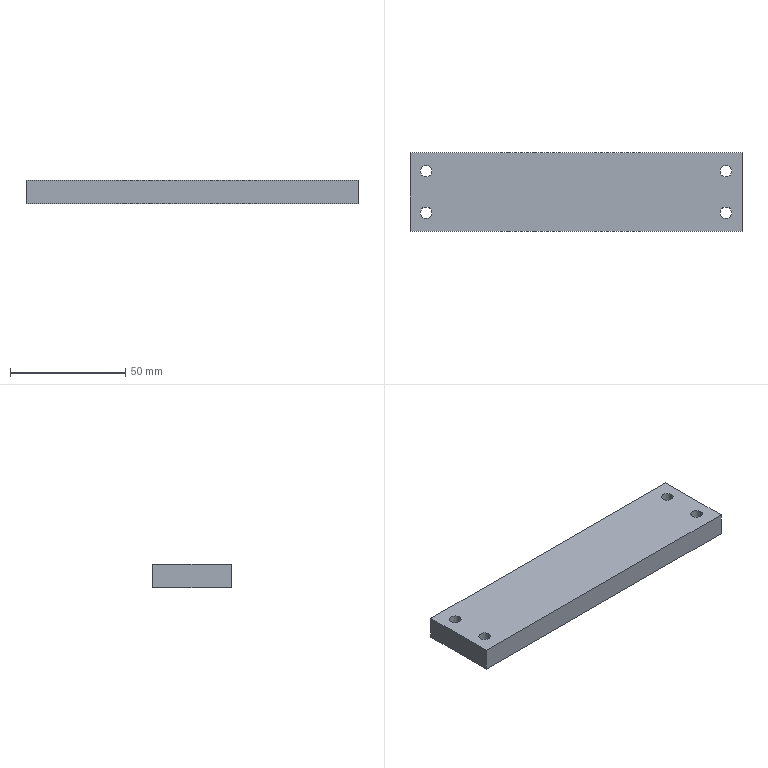Part | STEP file | Light curtain | 1 solid | 14 faces | box 144 x 34 x 10 mm | volume 48175 mm3 | cylinder 8 | plane 6 | commonest cylinder face diameters 5 x8
STEP:
#1=CARTESIAN_POINT('',(0.,0.,0.));
#2=DIRECTION('',(0.,0.,1.));
#3=DIRECTION('',(1.,0.,0.));
#4=AXIS2_PLACEMENT_3D('',#1,#2,#3);
#5=CARTESIAN_POINT('',(62.5,-9.,10.));
#6=VERTEX_POINT('',#5);
#7=CARTESIAN_POINT('',(62.5,-9.,0.));
#8=VERTEX_POINT('',#7);
#9=CARTESIAN_POINT('',(62.5,-9.,10.));
#10=DIRECTION('',(0.,0.,-1.));
#11=VECTOR('',#10,1.);
#12=LINE('',#9,#11);
#13=CARTESIAN_POINT('',(65.,-9.,10.));
#14=DIRECTION('',(0.,0.,-1.));
#15=DIRECTION('',(-1.,0.,0.));
#16=AXIS2_PLACEMENT_3D('',#13,#14,#15);
#17=CYLINDRICAL_SURFACE('',#16,2.5);
#18=CARTESIAN_POINT('',(6.283,0.));
#19=DIRECTION('',(0.,1.));
#20=VECTOR('',#19,1.);
#21=LINE('',#18,#20);
#22=(GEOMETRIC_REPRESENTATION_CONTEXT(2)PARAMETRIC_REPRESENTATION_CONTEXT()REPRESENTATION_CONTEXT('',''));
#23=DEFINITIONAL_REPRESENTATION('',(#21),#22);
#24=PCURVE('',#17,#23);
#25=CARTESIAN_POINT('',(65.,-9.,10.));
#26=DIRECTION('',(0.,0.,-1.));
#27=DIRECTION('',(-1.,0.,0.));
#28=AXIS2_PLACEMENT_3D('',#25,#26,#27);
#29=CYLINDRICAL_SURFACE('',#28,2.5);
#30=CARTESIAN_POINT('',(0.,0.));
#31=DIRECTION('',(0.,1.));
#32=VECTOR('',#31,1.);
#33=LINE('',#30,#32);
#34=(GEOMETRIC_REPRESENTATION_CONTEXT(2)PARAMETRIC_REPRESENTATION_CONTEXT()REPRESENTATION_CONTEXT('',''));
#35=DEFINITIONAL_REPRESENTATION('',(#33),#34);
#36=PCURVE('',#29,#35);
#37=SURFACE_CURVE('',#12,(#24,#36),.PCURVE_S1.);
#38=EDGE_CURVE('',#6,#8,#37,.T.);
#39=ORIENTED_EDGE('',*,*,#38,.T.);
#40=CARTESIAN_POINT('',(67.5,-9.,0.));
#41=VERTEX_POINT('',#40);
#42=CARTESIAN_POINT('',(65.,-9.,0.));
#43=DIRECTION('',(0.,0.,1.));
#44=DIRECTION('',(-1.,0.,0.));
#45=AXIS2_PLACEMENT_3D('',#42,#43,#44);
#46=CIRCLE('',#45,2.5);
#47=CARTESIAN_POINT('',(6.283,10.));
#48=DIRECTION('',(-1.,0.));
#49=VECTOR('',#48,1.);
#50=LINE('',#47,#49);
#51=(GEOMETRIC_REPRESENTATION_CONTEXT(2)PARAMETRIC_REPRESENTATION_CONTEXT()REPRESENTATION_CONTEXT('',''));
#52=DEFINITIONAL_REPRESENTATION('',(#50),#51);
#53=PCURVE('',#17,#52);
#54=CARTESIAN_POINT('',(72.,-17.,0.));
#55=DIRECTION('',(0.,0.,1.));
#56=DIRECTION('',(1.,0.,0.));
#57=AXIS2_PLACEMENT_3D('',#54,#55,#56);
#58=PLANE('',#57);
#59=CARTESIAN_POINT('',(-7.,8.));
#60=DIRECTION('',(-1.,0.));
#61=AXIS2_PLACEMENT_2D('',#59,#60);
#62=CIRCLE('',#61,2.5);
#63=(GEOMETRIC_REPRESENTATION_CONTEXT(2)PARAMETRIC_REPRESENTATION_CONTEXT()REPRESENTATION_CONTEXT('',''));
#64=DEFINITIONAL_REPRESENTATION('',(#62),#63);
#65=PCURVE('',#58,#64);
#66=SURFACE_CURVE('',#46,(#53,#65),.PCURVE_S1.);
#67=EDGE_CURVE('',#8,#41,#66,.T.);
#68=ORIENTED_EDGE('',*,*,#67,.T.);
#69=CARTESIAN_POINT('',(67.5,-9.,10.));
#70=VERTEX_POINT('',#69);
#71=CARTESIAN_POINT('',(67.5,-9.,10.));
#72=DIRECTION('',(0.,0.,-1.));
#73=VECTOR('',#72,1.);
#74=LINE('',#71,#73);
#75=CARTESIAN_POINT('',(3.142,0.));
#76=DIRECTION('',(0.,1.));
#77=VECTOR('',#76,1.);
#78=LINE('',#75,#77);
#79=(GEOMETRIC_REPRESENTATION_CONTEXT(2)PARAMETRIC_REPRESENTATION_CONTEXT()REPRESENTATION_CONTEXT('',''));
#80=DEFINITIONAL_REPRESENTATION('',(#78),#79);
#81=PCURVE('',#17,#80);
#82=CARTESIAN_POINT('',(3.142,0.));
#83=DIRECTION('',(0.,1.));
#84=VECTOR('',#83,1.);
#85=LINE('',#82,#84);
#86=(GEOMETRIC_REPRESENTATION_CONTEXT(2)PARAMETRIC_REPRESENTATION_CONTEXT()REPRESENTATION_CONTEXT('',''));
#87=DEFINITIONAL_REPRESENTATION('',(#85),#86);
#88=PCURVE('',#29,#87);
#89=SURFACE_CURVE('',#74,(#81,#88),.PCURVE_S1.);
#90=EDGE_CURVE('',#70,#41,#89,.T.);
#91=ORIENTED_EDGE('',*,*,#90,.F.);
#92=CARTESIAN_POINT('',(65.,-9.,10.));
#93=DIRECTION('',(0.,0.,-1.));
#94=DIRECTION('',(-1.,0.,0.));
#95=AXIS2_PLACEMENT_3D('',#92,#93,#94);
#96=CIRCLE('',#95,2.5);
#97=CARTESIAN_POINT('',(0.,0.));
#98=DIRECTION('',(1.,0.));
#99=VECTOR('',#98,1.);
#100=LINE('',#97,#99);
#101=(GEOMETRIC_REPRESENTATION_CONTEXT(2)PARAMETRIC_REPRESENTATION_CONTEXT()REPRESENTATION_CONTEXT('',''));
#102=DEFINITIONAL_REPRESENTATION('',(#100),#101);
#103=PCURVE('',#17,#102);
#104=CARTESIAN_POINT('',(72.,-17.,10.));
#105=DIRECTION('',(0.,0.,1.));
#106=DIRECTION('',(1.,0.,0.));
#107=AXIS2_PLACEMENT_3D('',#104,#105,#106);
#108=PLANE('',#107);
#109=CARTESIAN_POINT('',(-9.5,8.));
#110=CARTESIAN_POINT('',(-9.5,12.33));
#111=CARTESIAN_POINT('',(-5.75,10.165));
#112=CARTESIAN_POINT('',(-2.,8.));
#113=CARTESIAN_POINT('',(-5.75,5.835));
#114=CARTESIAN_POINT('',(-9.5,3.67));
#115=CARTESIAN_POINT('',(-9.5,8.));
#116=(BOUNDED_CURVE()B_SPLINE_CURVE(2,(#109,#110,#111,#112,#113,#114,#115),.UNSPECIFIED.,.T.,.F.)B_SPLINE_CURVE_WITH_KNOTS((1,2,2,2,2,1),(-2.094,0.,2.094,4.189,6.283,8.378),.UNSPECIFIED.)CURVE()GEOMETRIC_REPRESENTATION_ITEM()RATIONAL_B_SPLINE_CURVE((1.,0.5,1.,0.5,1.,0.5,1.))REPRESENTATION_ITEM(''));
#117=(GEOMETRIC_REPRESENTATION_CONTEXT(2)PARAMETRIC_REPRESENTATION_CONTEXT()REPRESENTATION_CONTEXT('',''));
#118=DEFINITIONAL_REPRESENTATION('',(#116),#117);
#119=PCURVE('',#108,#118);
#120=SURFACE_CURVE('',#96,(#103,#119),.PCURVE_S1.);
#121=EDGE_CURVE('',#70,#6,#120,.T.);
#122=ORIENTED_EDGE('',*,*,#121,.T.);
#123=EDGE_LOOP('',(#39,#68,#91,#122));
#124=FACE_BOUND('',#123,.F.);
#125=ADVANCED_FACE('',(#124),#17,.F.);
#126=CARTESIAN_POINT('',(62.5,9.,10.));
#127=VERTEX_POINT('',#126);
#128=CARTESIAN_POINT('',(62.5,9.,0.));
#129=VERTEX_POINT('',#128);
#130=CARTESIAN_POINT('',(62.5,9.,10.));
#131=DIRECTION('',(0.,0.,-1.));
#132=VECTOR('',#131,1.);
#133=LINE('',#130,#132);
#134=CARTESIAN_POINT('',(65.,9.,10.));
#135=DIRECTION('',(0.,0.,-1.));
#136=DIRECTION('',(-1.,0.,0.));
#137=AXIS2_PLACEMENT_3D('',#134,#135,#136);
#138=CYLINDRICAL_SURFACE('',#137,2.5);
#139=CARTESIAN_POINT('',(6.283,0.));
#140=DIRECTION('',(0.,1.));
#141=VECTOR('',#140,1.);
#142=LINE('',#139,#141);
#143=(GEOMETRIC_REPRESENTATION_CONTEXT(2)PARAMETRIC_REPRESENTATION_CONTEXT()REPRESENTATION_CONTEXT('',''));
#144=DEFINITIONAL_REPRESENTATION('',(#142),#143);
#145=PCURVE('',#138,#144);
#146=CARTESIAN_POINT('',(65.,9.,10.));
#147=DIRECTION('',(0.,0.,-1.));
#148=DIRECTION('',(-1.,0.,0.));
#149=AXIS2_PLACEMENT_3D('',#146,#147,#148);
#150=CYLINDRICAL_SURFACE('',#149,2.5);
#151=CARTESIAN_POINT('',(0.,0.));
#152=DIRECTION('',(0.,1.));
#153=VECTOR('',#152,1.);
#154=LINE('',#151,#153);
#155=(GEOMETRIC_REPRESENTATION_CONTEXT(2)PARAMETRIC_REPRESENTATION_CONTEXT()REPRESENTATION_CONTEXT('',''));
#156=DEFINITIONAL_REPRESENTATION('',(#154),#155);
#157=PCURVE('',#150,#156);
#158=SURFACE_CURVE('',#133,(#145,#157),.PCURVE_S1.);
#159=EDGE_CURVE('',#127,#129,#158,.T.);
#160=ORIENTED_EDGE('',*,*,#159,.T.);
#161=CARTESIAN_POINT('',(67.5,9.,0.));
#162=VERTEX_POINT('',#161);
#163=CARTESIAN_POINT('',(65.,9.,0.));
#164=DIRECTION('',(0.,0.,1.));
#165=DIRECTION('',(-1.,0.,0.));
#166=AXIS2_PLACEMENT_3D('',#163,#164,#165);
#167=CIRCLE('',#166,2.5);
#168=CARTESIAN_POINT('',(6.283,10.));
#169=DIRECTION('',(-1.,0.));
#170=VECTOR('',#169,1.);
#171=LINE('',#168,#170);
#172=(GEOMETRIC_REPRESENTATION_CONTEXT(2)PARAMETRIC_REPRESENTATION_CONTEXT()REPRESENTATION_CONTEXT('',''));
#173=DEFINITIONAL_REPRESENTATION('',(#171),#172);
#174=PCURVE('',#138,#173);
#175=CARTESIAN_POINT('',(-7.,26.));
#176=DIRECTION('',(-1.,0.));
#177=AXIS2_PLACEMENT_2D('',#175,#176);
#178=CIRCLE('',#177,2.5);
#179=(GEOMETRIC_REPRESENTATION_CONTEXT(2)PARAMETRIC_REPRESENTATION_CONTEXT()REPRESENTATION_CONTEXT('',''));
#180=DEFINITIONAL_REPRESENTATION('',(#178),#179);
#181=PCURVE('',#58,#180);
#182=SURFACE_CURVE('',#167,(#174,#181),.PCURVE_S1.);
#183=EDGE_CURVE('',#129,#162,#182,.T.);
#184=ORIENTED_EDGE('',*,*,#183,.T.);
#185=CARTESIAN_POINT('',(67.5,9.,10.));
#186=VERTEX_POINT('',#185);
#187=CARTESIAN_POINT('',(67.5,9.,10.));
#188=DIRECTION('',(0.,0.,-1.));
#189=VECTOR('',#188,1.);
#190=LINE('',#187,#189);
#191=CARTESIAN_POINT('',(3.142,0.));
#192=DIRECTION('',(0.,1.));
#193=VECTOR('',#192,1.);
#194=LINE('',#191,#193);
#195=(GEOMETRIC_REPRESENTATION_CONTEXT(2)PARAMETRIC_REPRESENTATION_CONTEXT()REPRESENTATION_CONTEXT('',''));
#196=DEFINITIONAL_REPRESENTATION('',(#194),#195);
#197=PCURVE('',#138,#196);
#198=CARTESIAN_POINT('',(3.142,0.));
#199=DIRECTION('',(0.,1.));
#200=VECTOR('',#199,1.);
#201=LINE('',#198,#200);
#202=(GEOMETRIC_REPRESENTATION_CONTEXT(2)PARAMETRIC_REPRESENTATION_CONTEXT()REPRESENTATION_CONTEXT('',''));
#203=DEFINITIONAL_REPRESENTATION('',(#201),#202);
#204=PCURVE('',#150,#203);
#205=SURFACE_CURVE('',#190,(#197,#204),.PCURVE_S1.);
#206=EDGE_CURVE('',#186,#162,#205,.T.);
#207=ORIENTED_EDGE('',*,*,#206,.F.);
#208=CARTESIAN_POINT('',(65.,9.,10.));
#209=DIRECTION('',(0.,0.,-1.));
#210=DIRECTION('',(-1.,0.,0.));
#211=AXIS2_PLACEMENT_3D('',#208,#209,#210);
#212=CIRCLE('',#211,2.5);
#213=CARTESIAN_POINT('',(0.,0.));
#214=DIRECTION('',(1.,0.));
#215=VECTOR('',#214,1.);
#216=LINE('',#213,#215);
#217=(GEOMETRIC_REPRESENTATION_CONTEXT(2)PARAMETRIC_REPRESENTATION_CONTEXT()REPRESENTATION_CONTEXT('',''));
#218=DEFINITIONAL_REPRESENTATION('',(#216),#217);
#219=PCURVE('',#138,#218);
#220=CARTESIAN_POINT('',(-9.5,26.));
#221=CARTESIAN_POINT('',(-9.5,30.33));
#222=CARTESIAN_POINT('',(-5.75,28.165));
#223=CARTESIAN_POINT('',(-2.,26.));
#224=CARTESIAN_POINT('',(-5.75,23.835));
#225=CARTESIAN_POINT('',(-9.5,21.67));
#226=CARTESIAN_POINT('',(-9.5,26.));
#227=(BOUNDED_CURVE()B_SPLINE_CURVE(2,(#220,#221,#222,#223,#224,#225,#226),.UNSPECIFIED.,.T.,.F.)B_SPLINE_CURVE_WITH_KNOTS((1,2,2,2,2,1),(-2.094,0.,2.094,4.189,6.283,8.378),.UNSPECIFIED.)CURVE()GEOMETRIC_REPRESENTATION_ITEM()RATIONAL_B_SPLINE_CURVE((1.,0.5,1.,0.5,1.,0.5,1.))REPRESENTATION_ITEM(''));
#228=(GEOMETRIC_REPRESENTATION_CONTEXT(2)PARAMETRIC_REPRESENTATION_CONTEXT()REPRESENTATION_CONTEXT('',''));
#229=DEFINITIONAL_REPRESENTATION('',(#227),#228);
#230=PCURVE('',#108,#229);
#231=SURFACE_CURVE('',#212,(#219,#230),.PCURVE_S1.);
#232=EDGE_CURVE('',#186,#127,#231,.T.);
#233=ORIENTED_EDGE('',*,*,#232,.T.);
#234=EDGE_LOOP('',(#160,#184,#207,#233));
#235=FACE_BOUND('',#234,.F.);
#236=ADVANCED_FACE('',(#235),#138,.F.);
#237=CARTESIAN_POINT('',(-67.5,-9.,10.));
#238=VERTEX_POINT('',#237);
#239=CARTESIAN_POINT('',(-67.5,-9.,0.));
#240=VERTEX_POINT('',#239);
#241=CARTESIAN_POINT('',(-67.5,-9.,10.));
#242=DIRECTION('',(0.,0.,-1.));
#243=VECTOR('',#242,1.);
#244=LINE('',#241,#243);
#245=CARTESIAN_POINT('',(-65.,-9.,10.));
#246=DIRECTION('',(0.,0.,-1.));
#247=DIRECTION('',(-1.,0.,0.));
#248=AXIS2_PLACEMENT_3D('',#245,#246,#247);
#249=CYLINDRICAL_SURFACE('',#248,2.5);
#250=CARTESIAN_POINT('',(6.283,0.));
#251=DIRECTION('',(0.,1.));
#252=VECTOR('',#251,1.);
#253=LINE('',#250,#252);
#254=(GEOMETRIC_REPRESENTATION_CONTEXT(2)PARAMETRIC_REPRESENTATION_CONTEXT()REPRESENTATION_CONTEXT('',''));
#255=DEFINITIONAL_REPRESENTATION('',(#253),#254);
#256=PCURVE('',#249,#255);
#257=CARTESIAN_POINT('',(-65.,-9.,10.));
#258=DIRECTION('',(0.,0.,-1.));
#259=DIRECTION('',(-1.,0.,0.));
#260=AXIS2_PLACEMENT_3D('',#257,#258,#259);
#261=CYLINDRICAL_SURFACE('',#260,2.5);
#262=CARTESIAN_POINT('',(0.,0.));
#263=DIRECTION('',(0.,1.));
#264=VECTOR('',#263,1.);
#265=LINE('',#262,#264);
#266=(GEOMETRIC_REPRESENTATION_CONTEXT(2)PARAMETRIC_REPRESENTATION_CONTEXT()REPRESENTATION_CONTEXT('',''));
#267=DEFINITIONAL_REPRESENTATION('',(#265),#266);
#268=PCURVE('',#261,#267);
#269=SURFACE_CURVE('',#244,(#256,#268),.PCURVE_S1.);
#270=EDGE_CURVE('',#238,#240,#269,.T.);
#271=ORIENTED_EDGE('',*,*,#270,.T.);
#272=CARTESIAN_POINT('',(-62.5,-9.,0.));
#273=VERTEX_POINT('',#272);
#274=CARTESIAN_POINT('',(-65.,-9.,0.));
#275=DIRECTION('',(0.,0.,1.));
#276=DIRECTION('',(-1.,0.,0.));
#277=AXIS2_PLACEMENT_3D('',#274,#275,#276);
#278=CIRCLE('',#277,2.5);
#279=CARTESIAN_POINT('',(6.283,10.));
#280=DIRECTION('',(-1.,0.));
#281=VECTOR('',#280,1.);
#282=LINE('',#279,#281);
#283=(GEOMETRIC_REPRESENTATION_CONTEXT(2)PARAMETRIC_REPRESENTATION_CONTEXT()REPRESENTATION_CONTEXT('',''));
#284=DEFINITIONAL_REPRESENTATION('',(#282),#283);
#285=PCURVE('',#249,#284);
#286=CARTESIAN_POINT('',(-137.,8.));
#287=DIRECTION('',(-1.,0.));
#288=AXIS2_PLACEMENT_2D('',#286,#287);
#289=CIRCLE('',#288,2.5);
#290=(GEOMETRIC_REPRESENTATION_CONTEXT(2)PARAMETRIC_REPRESENTATION_CONTEXT()REPRESENTATION_CONTEXT('',''));
#291=DEFINITIONAL_REPRESENTATION('',(#289),#290);
#292=PCURVE('',#58,#291);
#293=SURFACE_CURVE('',#278,(#285,#292),.PCURVE_S1.);
#294=EDGE_CURVE('',#240,#273,#293,.T.);
#295=ORIENTED_EDGE('',*,*,#294,.T.);
#296=CARTESIAN_POINT('',(-62.5,-9.,10.));
#297=VERTEX_POINT('',#296);
#298=CARTESIAN_POINT('',(-62.5,-9.,10.));
#299=DIRECTION('',(0.,0.,-1.));
#300=VECTOR('',#299,1.);
#301=LINE('',#298,#300);
#302=CARTESIAN_POINT('',(3.142,0.));
#303=DIRECTION('',(0.,1.));
#304=VECTOR('',#303,1.);
#305=LINE('',#302,#304);
#306=(GEOMETRIC_REPRESENTATION_CONTEXT(2)PARAMETRIC_REPRESENTATION_CONTEXT()REPRESENTATION_CONTEXT('',''));
#307=DEFINITIONAL_REPRESENTATION('',(#305),#306);
#308=PCURVE('',#249,#307);
#309=CARTESIAN_POINT('',(3.142,0.));
#310=DIRECTION('',(0.,1.));
#311=VECTOR('',#310,1.);
#312=LINE('',#309,#311);
#313=(GEOMETRIC_REPRESENTATION_CONTEXT(2)PARAMETRIC_REPRESENTATION_CONTEXT()REPRESENTATION_CONTEXT('',''));
#314=DEFINITIONAL_REPRESENTATION('',(#312),#313);
#315=PCURVE('',#261,#314);
#316=SURFACE_CURVE('',#301,(#308,#315),.PCURVE_S1.);
#317=EDGE_CURVE('',#297,#273,#316,.T.);
#318=ORIENTED_EDGE('',*,*,#317,.F.);
#319=CARTESIAN_POINT('',(-65.,-9.,10.));
#320=DIRECTION('',(0.,0.,-1.));
#321=DIRECTION('',(-1.,0.,0.));
#322=AXIS2_PLACEMENT_3D('',#319,#320,#321);
#323=CIRCLE('',#322,2.5);
#324=CARTESIAN_POINT('',(0.,0.));
#325=DIRECTION('',(1.,0.));
#326=VECTOR('',#325,1.);
#327=LINE('',#324,#326);
#328=(GEOMETRIC_REPRESENTATION_CONTEXT(2)PARAMETRIC_REPRESENTATION_CONTEXT()REPRESENTATION_CONTEXT('',''));
#329=DEFINITIONAL_REPRESENTATION('',(#327),#328);
#330=PCURVE('',#249,#329);
#331=CARTESIAN_POINT('',(-139.5,8.));
#332=CARTESIAN_POINT('',(-139.5,12.33));
#333=CARTESIAN_POINT('',(-135.75,10.165));
#334=CARTESIAN_POINT('',(-132.,8.));
#335=CARTESIAN_POINT('',(-135.75,5.835));
#336=CARTESIAN_POINT('',(-139.5,3.67));
#337=CARTESIAN_POINT('',(-139.5,8.));
#338=(BOUNDED_CURVE()B_SPLINE_CURVE(2,(#331,#332,#333,#334,#335,#336,#337),.UNSPECIFIED.,.T.,.F.)B_SPLINE_CURVE_WITH_KNOTS((1,2,2,2,2,1),(-2.094,0.,2.094,4.189,6.283,8.378),.UNSPECIFIED.)CURVE()GEOMETRIC_REPRESENTATION_ITEM()RATIONAL_B_SPLINE_CURVE((1.,0.5,1.,0.5,1.,0.5,1.))REPRESENTATION_ITEM(''));
#339=(GEOMETRIC_REPRESENTATION_CONTEXT(2)PARAMETRIC_REPRESENTATION_CONTEXT()REPRESENTATION_CONTEXT('',''));
#340=DEFINITIONAL_REPRESENTATION('',(#338),#339);
#341=PCURVE('',#108,#340);
#342=SURFACE_CURVE('',#323,(#330,#341),.PCURVE_S1.);
#343=EDGE_CURVE('',#297,#238,#342,.T.);
#344=ORIENTED_EDGE('',*,*,#343,.T.);
#345=EDGE_LOOP('',(#271,#295,#318,#344));
#346=FACE_BOUND('',#345,.F.);
#347=ADVANCED_FACE('',(#346),#249,.F.);
#348=CARTESIAN_POINT('',(-67.5,9.,10.));
#349=VERTEX_POINT('',#348);
#350=CARTESIAN_POINT('',(-67.5,9.,0.));
#351=VERTEX_POINT('',#350);
#352=CARTESIAN_POINT('',(-67.5,9.,10.));
#353=DIRECTION('',(0.,0.,-1.));
#354=VECTOR('',#353,1.);
#355=LINE('',#352,#354);
#356=CARTESIAN_POINT('',(-65.,9.,10.));
#357=DIRECTION('',(0.,0.,-1.));
#358=DIRECTION('',(-1.,0.,0.));
#359=AXIS2_PLACEMENT_3D('',#356,#357,#358);
#360=CYLINDRICAL_SURFACE('',#359,2.5);
#361=CARTESIAN_POINT('',(6.283,0.));
#362=DIRECTION('',(0.,1.));
#363=VECTOR('',#362,1.);
#364=LINE('',#361,#363);
#365=(GEOMETRIC_REPRESENTATION_CONTEXT(2)PARAMETRIC_REPRESENTATION_CONTEXT()REPRESENTATION_CONTEXT('',''));
#366=DEFINITIONAL_REPRESENTATION('',(#364),#365);
#367=PCURVE('',#360,#366);
#368=CARTESIAN_POINT('',(-65.,9.,10.));
#369=DIRECTION('',(0.,0.,-1.));
#370=DIRECTION('',(-1.,0.,0.));
#371=AXIS2_PLACEMENT_3D('',#368,#369,#370);
#372=CYLINDRICAL_SURFACE('',#371,2.5);
#373=CARTESIAN_POINT('',(0.,0.));
#374=DIRECTION('',(0.,1.));
#375=VECTOR('',#374,1.);
#376=LINE('',#373,#375);
#377=(GEOMETRIC_REPRESENTATION_CONTEXT(2)PARAMETRIC_REPRESENTATION_CONTEXT()REPRESENTATION_CONTEXT('',''));
#378=DEFINITIONAL_REPRESENTATION('',(#376),#377);
#379=PCURVE('',#372,#378);
#380=SURFACE_CURVE('',#355,(#367,#379),.PCURVE_S1.);
#381=EDGE_CURVE('',#349,#351,#380,.T.);
#382=ORIENTED_EDGE('',*,*,#381,.T.);
#383=CARTESIAN_POINT('',(-62.5,9.,0.));
#384=VERTEX_POINT('',#383);
#385=CARTESIAN_POINT('',(-65.,9.,0.));
#386=DIRECTION('',(0.,0.,1.));
#387=DIRECTION('',(-1.,0.,0.));
#388=AXIS2_PLACEMENT_3D('',#385,#386,#387);
#389=CIRCLE('',#388,2.5);
#390=CARTESIAN_POINT('',(6.283,10.));
#391=DIRECTION('',(-1.,0.));
#392=VECTOR('',#391,1.);
#393=LINE('',#390,#392);
#394=(GEOMETRIC_REPRESENTATION_CONTEXT(2)PARAMETRIC_REPRESENTATION_CONTEXT()REPRESENTATION_CONTEXT('',''));
#395=DEFINITIONAL_REPRESENTATION('',(#393),#394);
#396=PCURVE('',#360,#395);
#397=CARTESIAN_POINT('',(-137.,26.));
#398=DIRECTION('',(-1.,0.));
#399=AXIS2_PLACEMENT_2D('',#397,#398);
#400=CIRCLE('',#399,2.5);
#401=(GEOMETRIC_REPRESENTATION_CONTEXT(2)PARAMETRIC_REPRESENTATION_CONTEXT()REPRESENTATION_CONTEXT('',''));
#402=DEFINITIONAL_REPRESENTATION('',(#400),#401);
#403=PCURVE('',#58,#402);
#404=SURFACE_CURVE('',#389,(#396,#403),.PCURVE_S1.);
#405=EDGE_CURVE('',#351,#384,#404,.T.);
#406=ORIENTED_EDGE('',*,*,#405,.T.);
#407=CARTESIAN_POINT('',(-62.5,9.,10.));
#408=VERTEX_POINT('',#407);
#409=CARTESIAN_POINT('',(-62.5,9.,10.));
#410=DIRECTION('',(0.,0.,-1.));
#411=VECTOR('',#410,1.);
#412=LINE('',#409,#411);
#413=CARTESIAN_POINT('',(3.142,0.));
#414=DIRECTION('',(0.,1.));
#415=VECTOR('',#414,1.);
#416=LINE('',#413,#415);
#417=(GEOMETRIC_REPRESENTATION_CONTEXT(2)PARAMETRIC_REPRESENTATION_CONTEXT()REPRESENTATION_CONTEXT('',''));
#418=DEFINITIONAL_REPRESENTATION('',(#416),#417);
#419=PCURVE('',#360,#418);
#420=CARTESIAN_POINT('',(3.142,0.));
#421=DIRECTION('',(0.,1.));
#422=VECTOR('',#421,1.);
#423=LINE('',#420,#422);
#424=(GEOMETRIC_REPRESENTATION_CONTEXT(2)PARAMETRIC_REPRESENTATION_CONTEXT()REPRESENTATION_CONTEXT('',''));
#425=DEFINITIONAL_REPRESENTATION('',(#423),#424);
#426=PCURVE('',#372,#425);
#427=SURFACE_CURVE('',#412,(#419,#426),.PCURVE_S1.);
#428=EDGE_CURVE('',#408,#384,#427,.T.);
#429=ORIENTED_EDGE('',*,*,#428,.F.);
#430=CARTESIAN_POINT('',(-65.,9.,10.));
#431=DIRECTION('',(0.,0.,-1.));
#432=DIRECTION('',(-1.,0.,0.));
#433=AXIS2_PLACEMENT_3D('',#430,#431,#432);
#434=CIRCLE('',#433,2.5);
#435=CARTESIAN_POINT('',(0.,0.));
#436=DIRECTION('',(1.,0.));
#437=VECTOR('',#436,1.);
#438=LINE('',#435,#437);
#439=(GEOMETRIC_REPRESENTATION_CONTEXT(2)PARAMETRIC_REPRESENTATION_CONTEXT()REPRESENTATION_CONTEXT('',''));
#440=DEFINITIONAL_REPRESENTATION('',(#438),#439);
#441=PCURVE('',#360,#440);
#442=CARTESIAN_POINT('',(-139.5,26.));
#443=CARTESIAN_POINT('',(-139.5,30.33));
#444=CARTESIAN_POINT('',(-135.75,28.165));
#445=CARTESIAN_POINT('',(-132.,26.));
#446=CARTESIAN_POINT('',(-135.75,23.835));
#447=CARTESIAN_POINT('',(-139.5,21.67));
#448=CARTESIAN_POINT('',(-139.5,26.));
#449=(BOUNDED_CURVE()B_SPLINE_CURVE(2,(#442,#443,#444,#445,#446,#447,#448),.UNSPECIFIED.,.T.,.F.)B_SPLINE_CURVE_WITH_KNOTS((1,2,2,2,2,1),(-2.094,0.,2.094,4.189,6.283,8.378),.UNSPECIFIED.)CURVE()GEOMETRIC_REPRESENTATION_ITEM()RATIONAL_B_SPLINE_CURVE((1.,0.5,1.,0.5,1.,0.5,1.))REPRESENTATION_ITEM(''));
#450=(GEOMETRIC_REPRESENTATION_CONTEXT(2)PARAMETRIC_REPRESENTATION_CONTEXT()REPRESENTATION_CONTEXT('',''));
#451=DEFINITIONAL_REPRESENTATION('',(#449),#450);
#452=PCURVE('',#108,#451);
#453=SURFACE_CURVE('',#434,(#441,#452),.PCURVE_S1.);
#454=EDGE_CURVE('',#408,#349,#453,.T.);
#455=ORIENTED_EDGE('',*,*,#454,.T.);
#456=EDGE_LOOP('',(#382,#406,#429,#455));
#457=FACE_BOUND('',#456,.F.);
#458=ADVANCED_FACE('',(#457),#360,.F.);
#459=CARTESIAN_POINT('',(65.,-9.,10.));
#460=DIRECTION('',(0.,0.,-1.));
#461=DIRECTION('',(-1.,0.,0.));
#462=AXIS2_PLACEMENT_3D('',#459,#460,#461);
#463=CIRCLE('',#462,2.5);
#464=CARTESIAN_POINT('',(-9.5,8.));
#465=CARTESIAN_POINT('',(-9.5,12.33));
#466=CARTESIAN_POINT('',(-5.75,10.165));
#467=CARTESIAN_POINT('',(-2.,8.));
#468=CARTESIAN_POINT('',(-5.75,5.835));
#469=CARTESIAN_POINT('',(-9.5,3.67));
#470=CARTESIAN_POINT('',(-9.5,8.));
#471=(BOUNDED_CURVE()B_SPLINE_CURVE(2,(#464,#465,#466,#467,#468,#469,#470),.UNSPECIFIED.,.T.,.F.)B_SPLINE_CURVE_WITH_KNOTS((1,2,2,2,2,1),(-2.094,0.,2.094,4.189,6.283,8.378),.UNSPECIFIED.)CURVE()GEOMETRIC_REPRESENTATION_ITEM()RATIONAL_B_SPLINE_CURVE((1.,0.5,1.,0.5,1.,0.5,1.))REPRESENTATION_ITEM(''));
#472=(GEOMETRIC_REPRESENTATION_CONTEXT(2)PARAMETRIC_REPRESENTATION_CONTEXT()REPRESENTATION_CONTEXT('',''));
#473=DEFINITIONAL_REPRESENTATION('',(#471),#472);
#474=PCURVE('',#108,#473);
#475=CARTESIAN_POINT('',(0.,0.));
#476=DIRECTION('',(1.,0.));
#477=VECTOR('',#476,1.);
#478=LINE('',#475,#477);
#479=(GEOMETRIC_REPRESENTATION_CONTEXT(2)PARAMETRIC_REPRESENTATION_CONTEXT()REPRESENTATION_CONTEXT('',''));
#480=DEFINITIONAL_REPRESENTATION('',(#478),#479);
#481=PCURVE('',#29,#480);
#482=SURFACE_CURVE('',#463,(#474,#481),.PCURVE_S1.);
#483=EDGE_CURVE('',#6,#70,#482,.T.);
#484=ORIENTED_EDGE('',*,*,#483,.T.);
#485=ORIENTED_EDGE('',*,*,#121,.T.);
#486=EDGE_LOOP('',(#484,#485));
#487=FACE_BOUND('',#486,.T.);
#488=CARTESIAN_POINT('',(65.,9.,10.));
#489=DIRECTION('',(0.,0.,-1.));
#490=DIRECTION('',(-1.,0.,0.));
#491=AXIS2_PLACEMENT_3D('',#488,#489,#490);
#492=CIRCLE('',#491,2.5);
#493=CARTESIAN_POINT('',(-9.5,26.));
#494=CARTESIAN_POINT('',(-9.5,30.33));
#495=CARTESIAN_POINT('',(-5.75,28.165));
#496=CARTESIAN_POINT('',(-2.,26.));
#497=CARTESIAN_POINT('',(-5.75,23.835));
#498=CARTESIAN_POINT('',(-9.5,21.67));
#499=CARTESIAN_POINT('',(-9.5,26.));
#500=(BOUNDED_CURVE()B_SPLINE_CURVE(2,(#493,#494,#495,#496,#497,#498,#499),.UNSPECIFIED.,.T.,.F.)B_SPLINE_CURVE_WITH_KNOTS((1,2,2,2,2,1),(-2.094,0.,2.094,4.189,6.283,8.378),.UNSPECIFIED.)CURVE()GEOMETRIC_REPRESENTATION_ITEM()RATIONAL_B_SPLINE_CURVE((1.,0.5,1.,0.5,1.,0.5,1.))REPRESENTATION_ITEM(''));
#501=(GEOMETRIC_REPRESENTATION_CONTEXT(2)PARAMETRIC_REPRESENTATION_CONTEXT()REPRESENTATION_CONTEXT('',''));
#502=DEFINITIONAL_REPRESENTATION('',(#500),#501);
#503=PCURVE('',#108,#502);
#504=CARTESIAN_POINT('',(0.,0.));
#505=DIRECTION('',(1.,0.));
#506=VECTOR('',#505,1.);
#507=LINE('',#504,#506);
#508=(GEOMETRIC_REPRESENTATION_CONTEXT(2)PARAMETRIC_REPRESENTATION_CONTEXT()REPRESENTATION_CONTEXT('',''));
#509=DEFINITIONAL_REPRESENTATION('',(#507),#508);
#510=PCURVE('',#150,#509);
#511=SURFACE_CURVE('',#492,(#503,#510),.PCURVE_S1.);
#512=EDGE_CURVE('',#127,#186,#511,.T.);
#513=ORIENTED_EDGE('',*,*,#512,.T.);
#514=ORIENTED_EDGE('',*,*,#232,.T.);
#515=EDGE_LOOP('',(#513,#514));
#516=FACE_BOUND('',#515,.T.);
#517=CARTESIAN_POINT('',(-72.,17.,10.));
#518=VERTEX_POINT('',#517);
#519=CARTESIAN_POINT('',(-72.,-17.,10.));
#520=VERTEX_POINT('',#519);
#521=CARTESIAN_POINT('',(-72.,-17.,10.));
#522=DIRECTION('',(0.,-1.,0.));
#523=VECTOR('',#522,1.);
#524=LINE('',#521,#523);
#525=CARTESIAN_POINT('',(-144.,0.));
#526=DIRECTION('',(0.,-1.));
#527=VECTOR('',#526,1.);
#528=LINE('',#525,#527);
#529=(GEOMETRIC_REPRESENTATION_CONTEXT(2)PARAMETRIC_REPRESENTATION_CONTEXT()REPRESENTATION_CONTEXT('',''));
#530=DEFINITIONAL_REPRESENTATION('',(#528),#529);
#531=PCURVE('',#108,#530);
#532=CARTESIAN_POINT('',(-72.,17.,10.));
#533=DIRECTION('',(1.,0.,0.));
#534=DIRECTION('',(0.,0.,-1.));
#535=AXIS2_PLACEMENT_3D('',#532,#533,#534);
#536=PLANE('',#535);
#537=CARTESIAN_POINT('',(0.,-34.));
#538=DIRECTION('',(0.,-1.));
#539=VECTOR('',#538,1.);
#540=LINE('',#537,#539);
#541=(GEOMETRIC_REPRESENTATION_CONTEXT(2)PARAMETRIC_REPRESENTATION_CONTEXT()REPRESENTATION_CONTEXT('',''));
#542=DEFINITIONAL_REPRESENTATION('',(#540),#541);
#543=PCURVE('',#536,#542);
#544=SURFACE_CURVE('',#524,(#531,#543),.PCURVE_S1.);
#545=EDGE_CURVE('',#518,#520,#544,.T.);
#546=ORIENTED_EDGE('',*,*,#545,.T.);
#547=CARTESIAN_POINT('',(72.,-17.,10.));
#548=VERTEX_POINT('',#547);
#549=CARTESIAN_POINT('',(72.,-17.,10.));
#550=DIRECTION('',(1.,0.,0.));
#551=VECTOR('',#550,1.);
#552=LINE('',#549,#551);
#553=CARTESIAN_POINT('',(0.,0.));
#554=DIRECTION('',(1.,0.));
#555=VECTOR('',#554,1.);
#556=LINE('',#553,#555);
#557=(GEOMETRIC_REPRESENTATION_CONTEXT(2)PARAMETRIC_REPRESENTATION_CONTEXT()REPRESENTATION_CONTEXT('',''));
#558=DEFINITIONAL_REPRESENTATION('',(#556),#557);
#559=PCURVE('',#108,#558);
#560=CARTESIAN_POINT('',(-72.,-17.,10.));
#561=DIRECTION('',(0.,1.,0.));
#562=DIRECTION('',(0.,0.,1.));
#563=AXIS2_PLACEMENT_3D('',#560,#561,#562);
#564=PLANE('',#563);
#565=CARTESIAN_POINT('',(0.,144.));
#566=DIRECTION('',(0.,1.));
#567=VECTOR('',#566,1.);
#568=LINE('',#565,#567);
#569=(GEOMETRIC_REPRESENTATION_CONTEXT(2)PARAMETRIC_REPRESENTATION_CONTEXT()REPRESENTATION_CONTEXT('',''));
#570=DEFINITIONAL_REPRESENTATION('',(#568),#569);
#571=PCURVE('',#564,#570);
#572=SURFACE_CURVE('',#552,(#559,#571),.PCURVE_S1.);
#573=EDGE_CURVE('',#520,#548,#572,.T.);
#574=ORIENTED_EDGE('',*,*,#573,.T.);
#575=CARTESIAN_POINT('',(72.,17.,10.));
#576=VERTEX_POINT('',#575);
#577=CARTESIAN_POINT('',(72.,-17.,10.));
#578=DIRECTION('',(0.,1.,0.));
#579=VECTOR('',#578,1.);
#580=LINE('',#577,#579);
#581=CARTESIAN_POINT('',(0.,0.));
#582=DIRECTION('',(0.,1.));
#583=VECTOR('',#582,1.);
#584=LINE('',#581,#583);
#585=(GEOMETRIC_REPRESENTATION_CONTEXT(2)PARAMETRIC_REPRESENTATION_CONTEXT()REPRESENTATION_CONTEXT('',''));
#586=DEFINITIONAL_REPRESENTATION('',(#584),#585);
#587=PCURVE('',#108,#586);
#588=CARTESIAN_POINT('',(72.,17.,10.));
#589=DIRECTION('',(-1.,0.,0.));
#590=DIRECTION('',(0.,-1.,0.));
#591=AXIS2_PLACEMENT_3D('',#588,#589,#590);
#592=PLANE('',#591);
#593=CARTESIAN_POINT('',(34.,0.));
#594=DIRECTION('',(-1.,0.));
#595=VECTOR('',#594,1.);
#596=LINE('',#593,#595);
#597=(GEOMETRIC_REPRESENTATION_CONTEXT(2)PARAMETRIC_REPRESENTATION_CONTEXT()REPRESENTATION_CONTEXT('',''));
#598=DEFINITIONAL_REPRESENTATION('',(#596),#597);
#599=PCURVE('',#592,#598);
#600=SURFACE_CURVE('',#580,(#587,#599),.PCURVE_S1.);
#601=EDGE_CURVE('',#548,#576,#600,.T.);
#602=ORIENTED_EDGE('',*,*,#601,.T.);
#603=CARTESIAN_POINT('',(72.,17.,10.));
#604=DIRECTION('',(-1.,0.,0.));
#605=VECTOR('',#604,1.);
#606=LINE('',#603,#605);
#607=CARTESIAN_POINT('',(0.,34.));
#608=DIRECTION('',(-1.,0.));
#609=VECTOR('',#608,1.);
#610=LINE('',#607,#609);
#611=(GEOMETRIC_REPRESENTATION_CONTEXT(2)PARAMETRIC_REPRESENTATION_CONTEXT()REPRESENTATION_CONTEXT('',''));
#612=DEFINITIONAL_REPRESENTATION('',(#610),#611);
#613=PCURVE('',#108,#612);
#614=CARTESIAN_POINT('',(-72.,17.,10.));
#615=DIRECTION('',(0.,-1.,0.));
#616=DIRECTION('',(0.,0.,-1.));
#617=AXIS2_PLACEMENT_3D('',#614,#615,#616);
#618=PLANE('',#617);
#619=CARTESIAN_POINT('',(0.,144.));
#620=DIRECTION('',(0.,-1.));
#621=VECTOR('',#620,1.);
#622=LINE('',#619,#621);
#623=(GEOMETRIC_REPRESENTATION_CONTEXT(2)PARAMETRIC_REPRESENTATION_CONTEXT()REPRESENTATION_CONTEXT('',''));
#624=DEFINITIONAL_REPRESENTATION('',(#622),#623);
#625=PCURVE('',#618,#624);
#626=SURFACE_CURVE('',#606,(#613,#625),.PCURVE_S1.);
#627=EDGE_CURVE('',#576,#518,#626,.T.);
#628=ORIENTED_EDGE('',*,*,#627,.T.);
#629=EDGE_LOOP('',(#546,#574,#602,#628));
#630=FACE_BOUND('',#629,.T.);
#631=CARTESIAN_POINT('',(-65.,-9.,10.));
#632=DIRECTION('',(0.,0.,-1.));
#633=DIRECTION('',(-1.,0.,0.));
#634=AXIS2_PLACEMENT_3D('',#631,#632,#633);
#635=CIRCLE('',#634,2.5);
#636=CARTESIAN_POINT('',(-139.5,8.));
#637=CARTESIAN_POINT('',(-139.5,12.33));
#638=CARTESIAN_POINT('',(-135.75,10.165));
#639=CARTESIAN_POINT('',(-132.,8.));
#640=CARTESIAN_POINT('',(-135.75,5.835));
#641=CARTESIAN_POINT('',(-139.5,3.67));
#642=CARTESIAN_POINT('',(-139.5,8.));
#643=(BOUNDED_CURVE()B_SPLINE_CURVE(2,(#636,#637,#638,#639,#640,#641,#642),.UNSPECIFIED.,.T.,.F.)B_SPLINE_CURVE_WITH_KNOTS((1,2,2,2,2,1),(-2.094,0.,2.094,4.189,6.283,8.378),.UNSPECIFIED.)CURVE()GEOMETRIC_REPRESENTATION_ITEM()RATIONAL_B_SPLINE_CURVE((1.,0.5,1.,0.5,1.,0.5,1.))REPRESENTATION_ITEM(''));
#644=(GEOMETRIC_REPRESENTATION_CONTEXT(2)PARAMETRIC_REPRESENTATION_CONTEXT()REPRESENTATION_CONTEXT('',''));
#645=DEFINITIONAL_REPRESENTATION('',(#643),#644);
#646=PCURVE('',#108,#645);
#647=CARTESIAN_POINT('',(0.,0.));
#648=DIRECTION('',(1.,0.));
#649=VECTOR('',#648,1.);
#650=LINE('',#647,#649);
#651=(GEOMETRIC_REPRESENTATION_CONTEXT(2)PARAMETRIC_REPRESENTATION_CONTEXT()REPRESENTATION_CONTEXT('',''));
#652=DEFINITIONAL_REPRESENTATION('',(#650),#651);
#653=PCURVE('',#261,#652);
#654=SURFACE_CURVE('',#635,(#646,#653),.PCURVE_S1.);
#655=EDGE_CURVE('',#238,#297,#654,.T.);
#656=ORIENTED_EDGE('',*,*,#655,.T.);
#657=ORIENTED_EDGE('',*,*,#343,.T.);
#658=EDGE_LOOP('',(#656,#657));
#659=FACE_BOUND('',#658,.T.);
#660=CARTESIAN_POINT('',(-65.,9.,10.));
#661=DIRECTION('',(0.,0.,-1.));
#662=DIRECTION('',(-1.,0.,0.));
#663=AXIS2_PLACEMENT_3D('',#660,#661,#662);
#664=CIRCLE('',#663,2.5);
#665=CARTESIAN_POINT('',(-139.5,26.));
#666=CARTESIAN_POINT('',(-139.5,30.33));
#667=CARTESIAN_POINT('',(-135.75,28.165));
#668=CARTESIAN_POINT('',(-132.,26.));
#669=CARTESIAN_POINT('',(-135.75,23.835));
#670=CARTESIAN_POINT('',(-139.5,21.67));
#671=CARTESIAN_POINT('',(-139.5,26.));
#672=(BOUNDED_CURVE()B_SPLINE_CURVE(2,(#665,#666,#667,#668,#669,#670,#671),.UNSPECIFIED.,.T.,.F.)B_SPLINE_CURVE_WITH_KNOTS((1,2,2,2,2,1),(-2.094,0.,2.094,4.189,6.283,8.378),.UNSPECIFIED.)CURVE()GEOMETRIC_REPRESENTATION_ITEM()RATIONAL_B_SPLINE_CURVE((1.,0.5,1.,0.5,1.,0.5,1.))REPRESENTATION_ITEM(''));
#673=(GEOMETRIC_REPRESENTATION_CONTEXT(2)PARAMETRIC_REPRESENTATION_CONTEXT()REPRESENTATION_CONTEXT('',''));
#674=DEFINITIONAL_REPRESENTATION('',(#672),#673);
#675=PCURVE('',#108,#674);
#676=CARTESIAN_POINT('',(0.,0.));
#677=DIRECTION('',(1.,0.));
#678=VECTOR('',#677,1.);
#679=LINE('',#676,#678);
#680=(GEOMETRIC_REPRESENTATION_CONTEXT(2)PARAMETRIC_REPRESENTATION_CONTEXT()REPRESENTATION_CONTEXT('',''));
#681=DEFINITIONAL_REPRESENTATION('',(#679),#680);
#682=PCURVE('',#372,#681);
#683=SURFACE_CURVE('',#664,(#675,#682),.PCURVE_S1.);
#684=EDGE_CURVE('',#349,#408,#683,.T.);
#685=ORIENTED_EDGE('',*,*,#684,.T.);
#686=ORIENTED_EDGE('',*,*,#454,.T.);
#687=EDGE_LOOP('',(#685,#686));
#688=FACE_BOUND('',#687,.T.);
#689=ADVANCED_FACE('',(#487,#516,#630,#659,#688),#108,.T.);
#690=CARTESIAN_POINT('',(65.,-9.,0.));
#691=DIRECTION('',(0.,0.,1.));
#692=DIRECTION('',(-1.,0.,0.));
#693=AXIS2_PLACEMENT_3D('',#690,#691,#692);
#694=CIRCLE('',#693,2.5);
#695=CARTESIAN_POINT('',(6.283,10.));
#696=DIRECTION('',(-1.,0.));
#697=VECTOR('',#696,1.);
#698=LINE('',#695,#697);
#699=(GEOMETRIC_REPRESENTATION_CONTEXT(2)PARAMETRIC_REPRESENTATION_CONTEXT()REPRESENTATION_CONTEXT('',''));
#700=DEFINITIONAL_REPRESENTATION('',(#698),#699);
#701=PCURVE('',#29,#700);
#702=CARTESIAN_POINT('',(-7.,8.));
#703=DIRECTION('',(-1.,0.));
#704=AXIS2_PLACEMENT_2D('',#702,#703);
#705=CIRCLE('',#704,2.5);
#706=(GEOMETRIC_REPRESENTATION_CONTEXT(2)PARAMETRIC_REPRESENTATION_CONTEXT()REPRESENTATION_CONTEXT('',''));
#707=DEFINITIONAL_REPRESENTATION('',(#705),#706);
#708=PCURVE('',#58,#707);
#709=SURFACE_CURVE('',#694,(#701,#708),.PCURVE_S1.);
#710=EDGE_CURVE('',#41,#8,#709,.T.);
#711=ORIENTED_EDGE('',*,*,#710,.T.);
#712=ORIENTED_EDGE('',*,*,#38,.F.);
#713=ORIENTED_EDGE('',*,*,#483,.T.);
#714=ORIENTED_EDGE('',*,*,#90,.T.);
#715=EDGE_LOOP('',(#711,#712,#713,#714));
#716=FACE_BOUND('',#715,.F.);
#717=ADVANCED_FACE('',(#716),#29,.F.);
#718=CARTESIAN_POINT('',(65.,9.,0.));
#719=DIRECTION('',(0.,0.,1.));
#720=DIRECTION('',(-1.,0.,0.));
#721=AXIS2_PLACEMENT_3D('',#718,#719,#720);
#722=CIRCLE('',#721,2.5);
#723=CARTESIAN_POINT('',(6.283,10.));
#724=DIRECTION('',(-1.,0.));
#725=VECTOR('',#724,1.);
#726=LINE('',#723,#725);
#727=(GEOMETRIC_REPRESENTATION_CONTEXT(2)PARAMETRIC_REPRESENTATION_CONTEXT()REPRESENTATION_CONTEXT('',''));
#728=DEFINITIONAL_REPRESENTATION('',(#726),#727);
#729=PCURVE('',#150,#728);
#730=CARTESIAN_POINT('',(-7.,26.));
#731=DIRECTION('',(-1.,0.));
#732=AXIS2_PLACEMENT_2D('',#730,#731);
#733=CIRCLE('',#732,2.5);
#734=(GEOMETRIC_REPRESENTATION_CONTEXT(2)PARAMETRIC_REPRESENTATION_CONTEXT()REPRESENTATION_CONTEXT('',''));
#735=DEFINITIONAL_REPRESENTATION('',(#733),#734);
#736=PCURVE('',#58,#735);
#737=SURFACE_CURVE('',#722,(#729,#736),.PCURVE_S1.);
#738=EDGE_CURVE('',#162,#129,#737,.T.);
#739=ORIENTED_EDGE('',*,*,#738,.T.);
#740=ORIENTED_EDGE('',*,*,#159,.F.);
#741=ORIENTED_EDGE('',*,*,#512,.T.);
#742=ORIENTED_EDGE('',*,*,#206,.T.);
#743=EDGE_LOOP('',(#739,#740,#741,#742));
#744=FACE_BOUND('',#743,.F.);
#745=ADVANCED_FACE('',(#744),#150,.F.);
#746=CARTESIAN_POINT('',(72.,-17.,0.));
#747=VERTEX_POINT('',#746);
#748=CARTESIAN_POINT('',(72.,-17.,10.));
#749=DIRECTION('',(0.,0.,-1.));
#750=VECTOR('',#749,1.);
#751=LINE('',#748,#750);
#752=CARTESIAN_POINT('',(0.,144.));
#753=DIRECTION('',(-1.,0.));
#754=VECTOR('',#753,1.);
#755=LINE('',#752,#754);
#756=(GEOMETRIC_REPRESENTATION_CONTEXT(2)PARAMETRIC_REPRESENTATION_CONTEXT()REPRESENTATION_CONTEXT('',''));
#757=DEFINITIONAL_REPRESENTATION('',(#755),#756);
#758=PCURVE('',#564,#757);
#759=CARTESIAN_POINT('',(34.,0.));
#760=DIRECTION('',(0.,-1.));
#761=VECTOR('',#760,1.);
#762=LINE('',#759,#761);
#763=(GEOMETRIC_REPRESENTATION_CONTEXT(2)PARAMETRIC_REPRESENTATION_CONTEXT()REPRESENTATION_CONTEXT('',''));
#764=DEFINITIONAL_REPRESENTATION('',(#762),#763);
#765=PCURVE('',#592,#764);
#766=SURFACE_CURVE('',#751,(#758,#765),.PCURVE_S1.);
#767=EDGE_CURVE('',#548,#747,#766,.T.);
#768=ORIENTED_EDGE('',*,*,#767,.F.);
#769=ORIENTED_EDGE('',*,*,#573,.F.);
#770=CARTESIAN_POINT('',(-72.,-17.,0.));
#771=VERTEX_POINT('',#770);
#772=CARTESIAN_POINT('',(-72.,-17.,10.));
#773=DIRECTION('',(0.,0.,1.));
#774=VECTOR('',#773,1.);
#775=LINE('',#772,#774);
#776=CARTESIAN_POINT('',(0.,0.));
#777=DIRECTION('',(1.,0.));
#778=VECTOR('',#777,1.);
#779=LINE('',#776,#778);
#780=(GEOMETRIC_REPRESENTATION_CONTEXT(2)PARAMETRIC_REPRESENTATION_CONTEXT()REPRESENTATION_CONTEXT('',''));
#781=DEFINITIONAL_REPRESENTATION('',(#779),#780);
#782=PCURVE('',#564,#781);
#783=CARTESIAN_POINT('',(0.,-34.));
#784=DIRECTION('',(-1.,0.));
#785=VECTOR('',#784,1.);
#786=LINE('',#783,#785);
#787=(GEOMETRIC_REPRESENTATION_CONTEXT(2)PARAMETRIC_REPRESENTATION_CONTEXT()REPRESENTATION_CONTEXT('',''));
#788=DEFINITIONAL_REPRESENTATION('',(#786),#787);
#789=PCURVE('',#536,#788);
#790=SURFACE_CURVE('',#775,(#782,#789),.PCURVE_S1.);
#791=EDGE_CURVE('',#771,#520,#790,.T.);
#792=ORIENTED_EDGE('',*,*,#791,.F.);
#793=CARTESIAN_POINT('',(-72.,-17.,0.));
#794=DIRECTION('',(-1.,0.,0.));
#795=VECTOR('',#794,1.);
#796=LINE('',#793,#795);
#797=CARTESIAN_POINT('',(-10.,0.));
#798=DIRECTION('',(0.,-1.));
#799=VECTOR('',#798,1.);
#800=LINE('',#797,#799);
#801=(GEOMETRIC_REPRESENTATION_CONTEXT(2)PARAMETRIC_REPRESENTATION_CONTEXT()REPRESENTATION_CONTEXT('',''));
#802=DEFINITIONAL_REPRESENTATION('',(#800),#801);
#803=PCURVE('',#564,#802);
#804=CARTESIAN_POINT('',(-144.,0.));
#805=DIRECTION('',(-1.,0.));
#806=VECTOR('',#805,1.);
#807=LINE('',#804,#806);
#808=(GEOMETRIC_REPRESENTATION_CONTEXT(2)PARAMETRIC_REPRESENTATION_CONTEXT()REPRESENTATION_CONTEXT('',''));
#809=DEFINITIONAL_REPRESENTATION('',(#807),#808);
#810=PCURVE('',#58,#809);
#811=SURFACE_CURVE('',#796,(#803,#810),.PCURVE_S1.);
#812=EDGE_CURVE('',#747,#771,#811,.T.);
#813=ORIENTED_EDGE('',*,*,#812,.F.);
#814=EDGE_LOOP('',(#768,#769,#792,#813));
#815=FACE_BOUND('',#814,.T.);
#816=ADVANCED_FACE('',(#815),#564,.F.);
#817=ORIENTED_EDGE('',*,*,#791,.T.);
#818=ORIENTED_EDGE('',*,*,#545,.F.);
#819=CARTESIAN_POINT('',(-72.,17.,0.));
#820=VERTEX_POINT('',#819);
#821=CARTESIAN_POINT('',(-72.,17.,10.));
#822=DIRECTION('',(0.,0.,1.));
#823=VECTOR('',#822,1.);
#824=LINE('',#821,#823);
#825=CARTESIAN_POINT('',(0.,0.));
#826=DIRECTION('',(-1.,0.));
#827=VECTOR('',#826,1.);
#828=LINE('',#825,#827);
#829=(GEOMETRIC_REPRESENTATION_CONTEXT(2)PARAMETRIC_REPRESENTATION_CONTEXT()REPRESENTATION_CONTEXT('',''));
#830=DEFINITIONAL_REPRESENTATION('',(#828),#829);
#831=PCURVE('',#536,#830);
#832=CARTESIAN_POINT('',(0.,0.));
#833=DIRECTION('',(-1.,0.));
#834=VECTOR('',#833,1.);
#835=LINE('',#832,#834);
#836=(GEOMETRIC_REPRESENTATION_CONTEXT(2)PARAMETRIC_REPRESENTATION_CONTEXT()REPRESENTATION_CONTEXT('',''));
#837=DEFINITIONAL_REPRESENTATION('',(#835),#836);
#838=PCURVE('',#618,#837);
#839=SURFACE_CURVE('',#824,(#831,#838),.PCURVE_S1.);
#840=EDGE_CURVE('',#820,#518,#839,.T.);
#841=ORIENTED_EDGE('',*,*,#840,.F.);
#842=CARTESIAN_POINT('',(-72.,17.,0.));
#843=DIRECTION('',(0.,1.,0.));
#844=VECTOR('',#843,1.);
#845=LINE('',#842,#844);
#846=CARTESIAN_POINT('',(10.,0.));
#847=DIRECTION('',(0.,1.));
#848=VECTOR('',#847,1.);
#849=LINE('',#846,#848);
#850=(GEOMETRIC_REPRESENTATION_CONTEXT(2)PARAMETRIC_REPRESENTATION_CONTEXT()REPRESENTATION_CONTEXT('',''));
#851=DEFINITIONAL_REPRESENTATION('',(#849),#850);
#852=PCURVE('',#536,#851);
#853=CARTESIAN_POINT('',(-144.,34.));
#854=DIRECTION('',(0.,1.));
#855=VECTOR('',#854,1.);
#856=LINE('',#853,#855);
#857=(GEOMETRIC_REPRESENTATION_CONTEXT(2)PARAMETRIC_REPRESENTATION_CONTEXT()REPRESENTATION_CONTEXT('',''));
#858=DEFINITIONAL_REPRESENTATION('',(#856),#857);
#859=PCURVE('',#58,#858);
#860=SURFACE_CURVE('',#845,(#852,#859),.PCURVE_S1.);
#861=EDGE_CURVE('',#771,#820,#860,.T.);
#862=ORIENTED_EDGE('',*,*,#861,.F.);
#863=EDGE_LOOP('',(#817,#818,#841,#862));
#864=FACE_BOUND('',#863,.T.);
#865=ADVANCED_FACE('',(#864),#536,.F.);
#866=ORIENTED_EDGE('',*,*,#840,.T.);
#867=ORIENTED_EDGE('',*,*,#627,.F.);
#868=CARTESIAN_POINT('',(72.,17.,0.));
#869=VERTEX_POINT('',#868);
#870=CARTESIAN_POINT('',(72.,17.,10.));
#871=DIRECTION('',(0.,0.,1.));
#872=VECTOR('',#871,1.);
#873=LINE('',#870,#872);
#874=CARTESIAN_POINT('',(0.,144.));
#875=DIRECTION('',(-1.,0.));
#876=VECTOR('',#875,1.);
#877=LINE('',#874,#876);
#878=(GEOMETRIC_REPRESENTATION_CONTEXT(2)PARAMETRIC_REPRESENTATION_CONTEXT()REPRESENTATION_CONTEXT('',''));
#879=DEFINITIONAL_REPRESENTATION('',(#877),#878);
#880=PCURVE('',#618,#879);
#881=CARTESIAN_POINT('',(0.,0.));
#882=DIRECTION('',(0.,1.));
#883=VECTOR('',#882,1.);
#884=LINE('',#881,#883);
#885=(GEOMETRIC_REPRESENTATION_CONTEXT(2)PARAMETRIC_REPRESENTATION_CONTEXT()REPRESENTATION_CONTEXT('',''));
#886=DEFINITIONAL_REPRESENTATION('',(#884),#885);
#887=PCURVE('',#592,#886);
#888=SURFACE_CURVE('',#873,(#880,#887),.PCURVE_S1.);
#889=EDGE_CURVE('',#869,#576,#888,.T.);
#890=ORIENTED_EDGE('',*,*,#889,.F.);
#891=CARTESIAN_POINT('',(-72.,17.,0.));
#892=DIRECTION('',(1.,0.,0.));
#893=VECTOR('',#892,1.);
#894=LINE('',#891,#893);
#895=CARTESIAN_POINT('',(10.,0.));
#896=DIRECTION('',(0.,1.));
#897=VECTOR('',#896,1.);
#898=LINE('',#895,#897);
#899=(GEOMETRIC_REPRESENTATION_CONTEXT(2)PARAMETRIC_REPRESENTATION_CONTEXT()REPRESENTATION_CONTEXT('',''));
#900=DEFINITIONAL_REPRESENTATION('',(#898),#899);
#901=PCURVE('',#618,#900);
#902=CARTESIAN_POINT('',(-144.,34.));
#903=DIRECTION('',(1.,0.));
#904=VECTOR('',#903,1.);
#905=LINE('',#902,#904);
#906=(GEOMETRIC_REPRESENTATION_CONTEXT(2)PARAMETRIC_REPRESENTATION_CONTEXT()REPRESENTATION_CONTEXT('',''));
#907=DEFINITIONAL_REPRESENTATION('',(#905),#906);
#908=PCURVE('',#58,#907);
#909=SURFACE_CURVE('',#894,(#901,#908),.PCURVE_S1.);
#910=EDGE_CURVE('',#820,#869,#909,.T.);
#911=ORIENTED_EDGE('',*,*,#910,.F.);
#912=EDGE_LOOP('',(#866,#867,#890,#911));
#913=FACE_BOUND('',#912,.T.);
#914=ADVANCED_FACE('',(#913),#618,.F.);
#915=ORIENTED_EDGE('',*,*,#889,.T.);
#916=ORIENTED_EDGE('',*,*,#601,.F.);
#917=ORIENTED_EDGE('',*,*,#767,.T.);
#918=CARTESIAN_POINT('',(72.,17.,0.));
#919=DIRECTION('',(0.,-1.,0.));
#920=VECTOR('',#919,1.);
#921=LINE('',#918,#920);
#922=CARTESIAN_POINT('',(0.,-10.));
#923=DIRECTION('',(1.,0.));
#924=VECTOR('',#923,1.);
#925=LINE('',#922,#924);
#926=(GEOMETRIC_REPRESENTATION_CONTEXT(2)PARAMETRIC_REPRESENTATION_CONTEXT()REPRESENTATION_CONTEXT('',''));
#927=DEFINITIONAL_REPRESENTATION('',(#925),#926);
#928=PCURVE('',#592,#927);
#929=CARTESIAN_POINT('',(0.,34.));
#930=DIRECTION('',(0.,-1.));
#931=VECTOR('',#930,1.);
#932=LINE('',#929,#931);
#933=(GEOMETRIC_REPRESENTATION_CONTEXT(2)PARAMETRIC_REPRESENTATION_CONTEXT()REPRESENTATION_CONTEXT('',''));
#934=DEFINITIONAL_REPRESENTATION('',(#932),#933);
#935=PCURVE('',#58,#934);
#936=SURFACE_CURVE('',#921,(#928,#935),.PCURVE_S1.);
#937=EDGE_CURVE('',#869,#747,#936,.T.);
#938=ORIENTED_EDGE('',*,*,#937,.F.);
#939=EDGE_LOOP('',(#915,#916,#917,#938));
#940=FACE_BOUND('',#939,.T.);
#941=ADVANCED_FACE('',(#940),#592,.F.);
#942=CARTESIAN_POINT('',(-65.,-9.,0.));
#943=DIRECTION('',(0.,0.,1.));
#944=DIRECTION('',(-1.,0.,0.));
#945=AXIS2_PLACEMENT_3D('',#942,#943,#944);
#946=CIRCLE('',#945,2.5);
#947=CARTESIAN_POINT('',(6.283,10.));
#948=DIRECTION('',(-1.,0.));
#949=VECTOR('',#948,1.);
#950=LINE('',#947,#949);
#951=(GEOMETRIC_REPRESENTATION_CONTEXT(2)PARAMETRIC_REPRESENTATION_CONTEXT()REPRESENTATION_CONTEXT('',''));
#952=DEFINITIONAL_REPRESENTATION('',(#950),#951);
#953=PCURVE('',#261,#952);
#954=CARTESIAN_POINT('',(-137.,8.));
#955=DIRECTION('',(-1.,0.));
#956=AXIS2_PLACEMENT_2D('',#954,#955);
#957=CIRCLE('',#956,2.5);
#958=(GEOMETRIC_REPRESENTATION_CONTEXT(2)PARAMETRIC_REPRESENTATION_CONTEXT()REPRESENTATION_CONTEXT('',''));
#959=DEFINITIONAL_REPRESENTATION('',(#957),#958);
#960=PCURVE('',#58,#959);
#961=SURFACE_CURVE('',#946,(#953,#960),.PCURVE_S1.);
#962=EDGE_CURVE('',#273,#240,#961,.T.);
#963=ORIENTED_EDGE('',*,*,#962,.T.);
#964=ORIENTED_EDGE('',*,*,#270,.F.);
#965=ORIENTED_EDGE('',*,*,#655,.T.);
#966=ORIENTED_EDGE('',*,*,#317,.T.);
#967=EDGE_LOOP('',(#963,#964,#965,#966));
#968=FACE_BOUND('',#967,.F.);
#969=ADVANCED_FACE('',(#968),#261,.F.);
#970=CARTESIAN_POINT('',(-65.,9.,0.));
#971=DIRECTION('',(0.,0.,1.));
#972=DIRECTION('',(-1.,0.,0.));
#973=AXIS2_PLACEMENT_3D('',#970,#971,#972);
#974=CIRCLE('',#973,2.5);
#975=CARTESIAN_POINT('',(6.283,10.));
#976=DIRECTION('',(-1.,0.));
#977=VECTOR('',#976,1.);
#978=LINE('',#975,#977);
#979=(GEOMETRIC_REPRESENTATION_CONTEXT(2)PARAMETRIC_REPRESENTATION_CONTEXT()REPRESENTATION_CONTEXT('',''));
#980=DEFINITIONAL_REPRESENTATION('',(#978),#979);
#981=PCURVE('',#372,#980);
#982=CARTESIAN_POINT('',(-137.,26.));
#983=DIRECTION('',(-1.,0.));
#984=AXIS2_PLACEMENT_2D('',#982,#983);
#985=CIRCLE('',#984,2.5);
#986=(GEOMETRIC_REPRESENTATION_CONTEXT(2)PARAMETRIC_REPRESENTATION_CONTEXT()REPRESENTATION_CONTEXT('',''));
#987=DEFINITIONAL_REPRESENTATION('',(#985),#986);
#988=PCURVE('',#58,#987);
#989=SURFACE_CURVE('',#974,(#981,#988),.PCURVE_S1.);
#990=EDGE_CURVE('',#384,#351,#989,.T.);
#991=ORIENTED_EDGE('',*,*,#990,.T.);
#992=ORIENTED_EDGE('',*,*,#381,.F.);
#993=ORIENTED_EDGE('',*,*,#684,.T.);
#994=ORIENTED_EDGE('',*,*,#428,.T.);
#995=EDGE_LOOP('',(#991,#992,#993,#994));
#996=FACE_BOUND('',#995,.F.);
#997=ADVANCED_FACE('',(#996),#372,.F.);
#998=ORIENTED_EDGE('',*,*,#67,.T.);
#999=ORIENTED_EDGE('',*,*,#710,.T.);
#1000=EDGE_LOOP('',(#998,#999));
#1001=FACE_BOUND('',#1000,.T.);
#1002=ORIENTED_EDGE('',*,*,#183,.T.);
#1003=ORIENTED_EDGE('',*,*,#738,.T.);
#1004=EDGE_LOOP('',(#1002,#1003));
#1005=FACE_BOUND('',#1004,.T.);
#1006=ORIENTED_EDGE('',*,*,#812,.T.);
#1007=ORIENTED_EDGE('',*,*,#861,.T.);
#1008=ORIENTED_EDGE('',*,*,#910,.T.);
#1009=ORIENTED_EDGE('',*,*,#937,.T.);
#1010=EDGE_LOOP('',(#1006,#1007,#1008,#1009));
#1011=FACE_BOUND('',#1010,.T.);
#1012=ORIENTED_EDGE('',*,*,#294,.T.);
#1013=ORIENTED_EDGE('',*,*,#962,.T.);
#1014=EDGE_LOOP('',(#1012,#1013));
#1015=FACE_BOUND('',#1014,.T.);
#1016=ORIENTED_EDGE('',*,*,#405,.T.);
#1017=ORIENTED_EDGE('',*,*,#990,.T.);
#1018=EDGE_LOOP('',(#1016,#1017));
#1019=FACE_BOUND('',#1018,.T.);
#1020=ADVANCED_FACE('',(#1001,#1005,#1011,#1015,#1019),#58,.F.);
#1021=CLOSED_SHELL('',(#125,#236,#347,#458,#689,#717,#745,#816,#865,#914,#941,#969,#997,#1020));
#1022=MANIFOLD_SOLID_BREP('',#1021);
#1023=(LENGTH_UNIT()NAMED_UNIT(*)SI_UNIT(.MILLI.,.METRE.));
#1024=UNCERTAINTY_MEASURE_WITH_UNIT(LENGTH_MEASURE(0.0000001),#1023,'','');
#1025=(NAMED_UNIT(*)PLANE_ANGLE_UNIT()SI_UNIT($,.RADIAN.));
#1026=(NAMED_UNIT(*)SI_UNIT($,.STERADIAN.)SOLID_ANGLE_UNIT());
#1027=(GEOMETRIC_REPRESENTATION_CONTEXT(3)GLOBAL_UNCERTAINTY_ASSIGNED_CONTEXT((#1024))GLOBAL_UNIT_ASSIGNED_CONTEXT((#1023,#1025,#1026))REPRESENTATION_CONTEXT('',''));
#1028=ADVANCED_BREP_SHAPE_REPRESENTATION('',(#4,#1022),#1027);